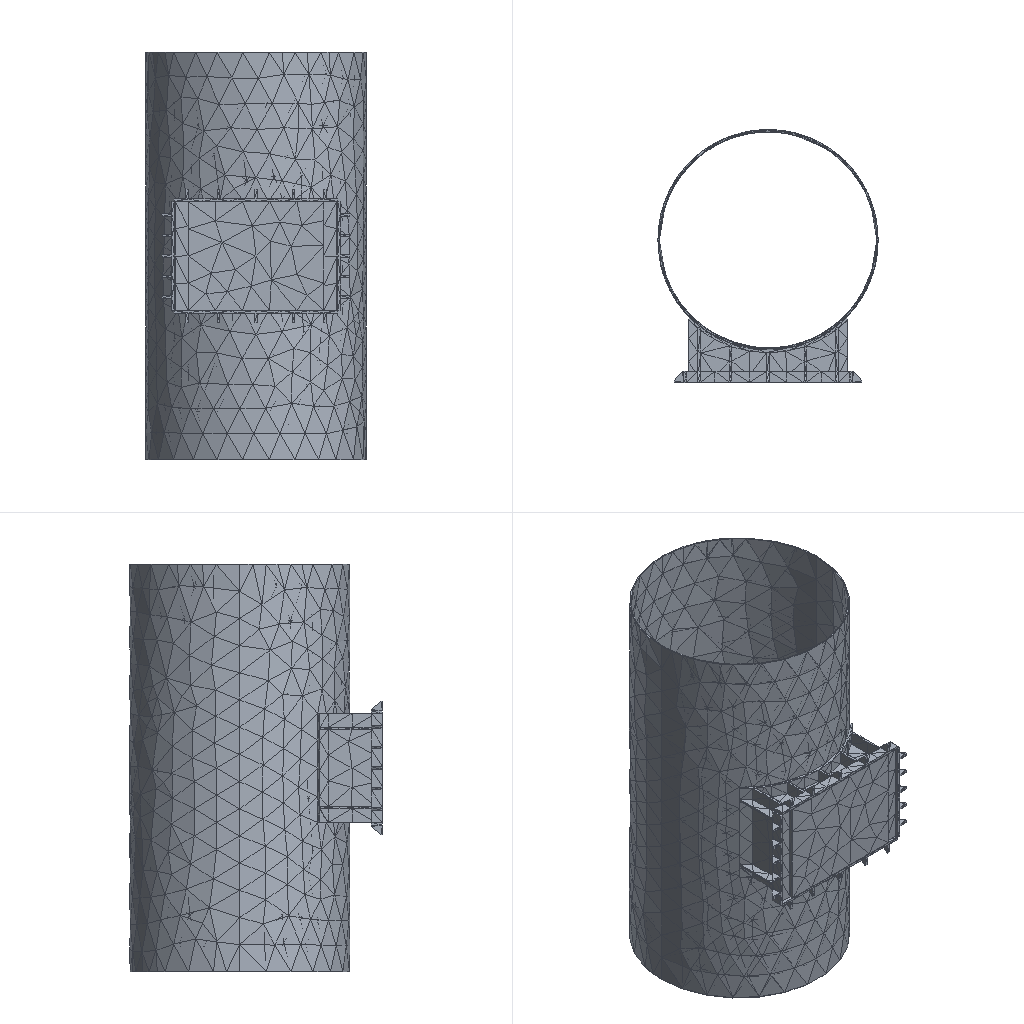Simulation study | ansys workbench
Set-up summary:
category,name,step,type,value,unit,region
solver,ansys_workbench
units,mm-N-s-tonne (MPa),,stated,"/units,MPA"
analysis,LS1,,static
load_step,LS1,LS1,static,nsubst=1; time=1
mesh,nodes,,,10077
mesh,elements,,,5774
element_type,SOLID187,,,4979
element_type,SURF154,,,571
element_type,TARGE170,,,112
element_type,CONTA174,,,112
material,q355,,E,200000,tonne s^-2 mm^-1
material,q355,,nu,0.3
material,q355,,density,7.85e-09,tonne mm^-3
material,q355,,conductivity,60.5,tonne mm s^-3 C^-1
material,q355,,specific_heat,4.34e+08,mm^2 s^-2 C^-1
material,q355,,cte,1.2e-05,C^-1
material,q355,,permeability,10000
material,q355,,resistivity,0.00017,ohm mm
load,Define Force Using Surface Effect Elements,LS1,surface-effect pres face 1,3.026,,SURF154 #8
load,Define Force Using Surface Effect Elements,LS1,surface-effect pres face 1,-3.026,,SURF154 #9
load,Define Force Using Surface Effect Elements,LS1,surface-effect pres face 2,-0.146,,SURF154 #10
load,Define Force Using Surface Effect Elements,LS1,surface-effect pres face 2,3.162,,SURF154 #11
load,Define Force Using Surface Effect Elements,LS1,surface-effect pres face 3,-1.925,,SURF154 #12
bc,Fixed Supports,model,fixed,[dofs=ALL],,_FIXEDSU
contact,Contact Region,,bonded (always),element=CONTA174
contact,Contact Region 2,,bonded (always),element=CONTA174
named_set,_FIXEDSU,,node,463
Ansys APDL input file, long lists of numbers shortened:
/batch
/config,noeldb,1     ! force off writing results to database
*get,_wallstrt,active,,time,wall
! ANSYS input file written by Workbench version 2022 R1
! File used for geometry attach:
/title,111--____ (B5)
! ****** Begin Custom Load Command Snippet ******
/COM, ACT Extensions:
/COM,     LSDYNA, 2021.1
/COM,
! ****** End   Custom Load Command Snippet ******
*DIM,_wb_ProjectScratch_dir,string,248
_wb_ProjectScratch_dir(1) = ''
*DIM,_wb_SolverFiles_dir,string,248
_wb_SolverFiles_dir(1) = ''
*DIM,_wb_userfiles_dir,string,248
_wb_userfiles_dir(1) = ''
/com,--- Data in consistent NMM units. See Solving Units in the help system for more information.
/units,MPA
/nopr
/wb,file,start              !  signify a WB generated input file
/prep7
! Turn off shape checking because checks already performed inside WB mesher.
! See help system for more information.
SHPP,OFF,,NOWARN
/nolist
etcon,set             ! allow ANSYS to choose best KEYOP's for 180x elements, resets any applicable keyopt to MAPDL defaults
/com,*********** Nodes for the whole assembly ***********
nblock,3,,11084
(1i9,3e20.9e3)
        1    -5.150000000E+02    -9.680000000E+02     4.200000000E+02
! (10076 more lines like these left out)
-1
/wb,elem,start            !  set before creation of elements
/com,*********** Elements for Body 1 "1-FreeParts|NONE" ***********
et,1,187
eblock,19,solid,,4736
(19i9)
        1        1        1        1        0        0        0        0       10        0      244     1292     2139     2144     1297     5916     9964     5917     5913
! (9471 more lines like these left out)
-1
/com,*********** Elements for Body 2 "1-FreeParts|__-__3" ***********
et,2,187
eblock,19,solid,,119
(19i9)
        2        2        2        2        0        0        0        0       10        0        1       12       14       65       16      149      170      154      150
! (237 more lines like these left out)
-1
/com,*********** Elements for Body 3 "1-FreeParts|__2" ***********
et,3,187
eblock,19,solid,,124
(19i9)
        3        3        3        3        0        0        0        0       10        0      120      363      411      410      419      523      687      522      524
! (247 more lines like these left out)
-1
/wb,elem,end               !  done creating elements
/com,*********** Send User Defined Coordinate System(s) ***********
csys,0
toffst,273.15,  ! Temperature offset from absolute zero
/com,*********** Set Reference Temperature ***********
tref,22.
/wb,mat,start              !  starting to send materials
/com,*********** Send Materials ***********
Temperature = 'TEMP' ! Temperature
MP,DENS,1,7.85e-09,	! tonne mm^-3
MP,ALPX,1,1.2e-05,	! C^-1
MP,C,1,434000000,	! mm^2 s^-2 C^-1
MP,KXX,1,60.5,	! tonne mm s^-3 C^-1
MP,RSVX,1,0.00017,	! ohm mm
MP,EX,1,200000,	! tonne s^-2 mm^-1
MP,NUXY,1,0.3,
MP,MURX,1,10000,
Temperature = 'TEMP' ! Temperature
MP,DENS,2,7.85e-09,	! tonne mm^-3
MP,ALPX,2,1.2e-05,	! C^-1
MP,C,2,434000000,	! mm^2 s^-2 C^-1
MP,KXX,2,60.5,	! tonne mm s^-3 C^-1
MP,RSVX,2,0.00017,	! ohm mm
MP,EX,2,200000,	! tonne s^-2 mm^-1
MP,NUXY,2,0.3,
MP,MURX,2,10000,
Temperature = 'TEMP' ! Temperature
MP,DENS,3,7.85e-09,	! tonne mm^-3
MP,ALPX,3,1.2e-05,	! C^-1
MP,C,3,434000000,	! mm^2 s^-2 C^-1
MP,KXX,3,60.5,	! tonne mm s^-3 C^-1
MP,RSVX,3,0.00017,	! ohm mm
MP,EX,3,200000,	! tonne s^-2 mm^-1
MP,NUXY,3,0.3,
MP,MURX,3,10000,
/wb,mat,end                !  done sending materials
!************************* Model Summary ********************
!1-FreeParts|NONE,	q355,	matid,	1
!1-FreeParts|__-__3,	q355,	matid,	2
!1-FreeParts|__2,	q355,	matid,	3
!************************* End Model Summary ********************
! get the diagonal of the bounding box. Needed later for other things
*get,_xmin,node,,mnloc,x
*get,_ymin,node,,mnloc,y
*get,_zmin,node,,mnloc,z
*get,_xmax,node,,mxloc,x
*get,_ymax,node,,mxloc,y
*get,_zmax,node,,mxloc,z
_ASMDIAG=(_xmax-_xmin)*(_xmax-_xmin)+(_ymax-_ymin)*(_ymax-_ymin)+(_zmax-_zmin)*(_zmax-_zmin)
_ASMDIAG=SQRT(_ASMDIAG)
/wb,contact,start          !  starting to send contact
/com,*********** Create Contact "接触区域" ***********
/com,            Real Constant Set For Above Contact Is 5 & 4
*set,tid,5
*set,cid,4
r,tid
r,cid
et,tid,170
et,cid,174
eblock,10,,,44
(15i9)
     8264        5        5        5        0      842     1090      874      874     3213     3332      874     3212
! (43 more lines like these left out)
-1
eblock,10,,,44
(15i9)
     8308        4        4        4        0      842     1090      874      874     3213     3332      874     3212
! (43 more lines like these left out)
-1
eblock,10,,,12
(15i9)
     8352        4        5        4        0       30       27       66       66      241      242       66      251
! (11 more lines like these left out)
-1
eblock,10,,,12
(15i9)
     8364        5        4        5        0       30       27       66       66      241      242       66      251
! (11 more lines like these left out)
-1
keyo,cid,8,2               ! auto create asymmetric contact (from Program Controlled setting)
keyo,cid,10,0              ! adjust contact stiffness each NR iteration (from Program Controlled setting)
keyo,cid,12,5              ! bonded always
keyo,cid,18,1              ! small sliding turned on by application
keyo,cid,2,0               ! augmented Lagrange (from Program Controlled setting)
keyo,cid,4,0               ! on Gauss point (from Program Controlled setting)
keyo,cid,9,1               ! ignore initial gaps/penetration
keyo,cid,7,0               ! No Prediction
rmod,tid,3,10.      ! FKN
rmod,tid,5,0.       ! ICONT
rmod,tid,6,0.       ! PINB
rmod,tid,10,0.      ! CNOF
rmod,tid,12,0.      ! FKT
rmod,tid,36,32      ! WB DSID
rmod,cid,3,10.      ! FKN
rmod,cid,5,0.       ! ICONT
rmod,cid,6,0.       ! PINB
rmod,cid,10,0.      ! CNOF
rmod,cid,12,0.      ! FKT
rmod,cid,36,32      ! WB DSID
/com,*********** Create Contact "接触区域 2" ***********
/com,            Real Constant Set For Above Contact Is 7 & 6
*set,tid,7
*set,cid,6
r,tid
r,cid
et,tid,170
et,cid,174
eblock,10,,,44
(15i9)
     8376        7        7        7        0      877     1199     1110     1110     3359     5061     1110     3358
! (43 more lines like these left out)
-1
eblock,10,,,44
(15i9)
     8420        6        6        6        0      877     1199     1110     1110     3359     5061     1110     3358
! (43 more lines like these left out)
-1
eblock,10,,,12
(15i9)
     8464        6        7        6        0      375      378      402      402      590      600      402      591
! (11 more lines like these left out)
-1
eblock,10,,,12
(15i9)
     8476        7        6        7        0      375      378      402      402      590      600      402      591
! (11 more lines like these left out)
-1
keyo,cid,8,2               ! auto create asymmetric contact (from Program Controlled setting)
keyo,cid,10,0              ! adjust contact stiffness each NR iteration (from Program Controlled setting)
keyo,cid,12,5              ! bonded always
keyo,cid,18,1              ! small sliding turned on by application
keyo,cid,2,0               ! augmented Lagrange (from Program Controlled setting)
keyo,cid,4,0               ! on Gauss point (from Program Controlled setting)
keyo,cid,9,1               ! ignore initial gaps/penetration
keyo,cid,7,0               ! No Prediction
rmod,tid,3,10.      ! FKN
rmod,tid,5,0.       ! ICONT
rmod,tid,6,0.       ! PINB
rmod,tid,10,0.      ! CNOF
rmod,tid,12,0.      ! FKT
rmod,tid,36,35      ! WB DSID
rmod,cid,3,10.      ! FKN
rmod,cid,5,0.       ! ICONT
rmod,cid,6,0.       ! PINB
rmod,cid,10,0.      ! CNOF
rmod,cid,12,0.      ! FKT
rmod,cid,36,35      ! WB DSID
nsel,all
esel,all
/wb,contact,end            !  done creating contacts
/golist
/wb,load,start             !  starting to send loads
/com,*********** Fixed Supports ***********
CMBLOCK,_FIXEDSU,NODE,      463
(8i10)
         2         4         5         7         8        11        13        14
! (57 more lines like these left out)
cmsel,s,_FIXEDSU
d,all,all
nsel,all
/com,*********** Define Force Using Surface Effect Elements ***********
local,12,0,0.,0.,0.,0.,0.,0.
csys,0
et,8,154
eblock,10,,,14
(15i9)
     8488        8        8        8       12     1100     2154     2153     2153     5015     9987     2153     5014
! (13 more lines like these left out)
-1
esel,s,type,,8
keyop,8,2,1                ! Apply load in local coordinate system
keyop,8,7,1                ! Use original area so load is constant in large deformation
esel,all
/com,*********** Define Force Using Surface Effect Elements ***********
local,13,0,0.,0.,0.,0.,0.,0.
csys,0
et,9,154
eblock,10,,,14
(15i9)
     8502        9        9        9       13     1079     1080     2151     2151     4860     4877     2151     4866
! (13 more lines like these left out)
-1
esel,s,type,,9
keyop,9,2,1                ! Apply load in local coordinate system
keyop,9,7,1                ! Use original area so load is constant in large deformation
esel,all
/com,*********** Define Force Using Surface Effect Elements ***********
local,14,0,0.,0.,0.,0.,0.,0.
csys,0
et,10,154
eblock,10,,,437
(15i9)
     8516       10       10       10       14      718     2089      732      732     2364     2500      732     2361
! (436 more lines like these left out)
-1
esel,s,type,,10
keyop,10,2,1                ! Apply load in local coordinate system
keyop,10,7,1                ! Use original area so load is constant in large deformation
esel,all
/com,*********** Define Force Using Surface Effect Elements ***********
local,15,0,0.,0.,0.,0.,0.,0.
csys,0
et,11,154
eblock,10,,,74
(15i9)
     8953       11       11       11       15     1372     1105     1101     1101     5040     5017     1101     5020
! (73 more lines like these left out)
-1
esel,s,type,,11
keyop,11,2,1                ! Apply load in local coordinate system
keyop,11,7,1                ! Use original area so load is constant in large deformation
esel,all
/com,*********** Define Force Using Surface Effect Elements ***********
local,16,0,0.,0.,0.,0.,0.,0.
csys,0
et,12,154
eblock,10,,,32
(15i9)
     9027       12       12       12       16      994     1023     1043     1043     4343     4541     1043     4344
! (31 more lines like these left out)
-1
esel,s,type,,12
keyop,12,2,1                ! Apply load in local coordinate system
keyop,12,7,1                ! Use original area so load is constant in large deformation
esel,all
/gst,on,on
fini
*get,_numnode,node,0,count
*get,_numelem,elem,0,count
*get, _MAXELEMNUM, elem, 0, NUM, MAX
*get, _MAXNODENUM, node, 0, NUM, MAX
*get, _MAXELEMTYPE, etyp, 0, NUM, MAX
*get, _MAXREALCONST, real, 0, NUM, MAX
/go
/wb,load,end               !  done creating loads
/com,--- Number of total nodes = %_numnode%
/com,--- Number of contact elements = 795
/com,--- Number of spring elements = 0
/com,--- Number of bearing elements = 0
/com,--- Number of solid elements = 4979
/com,--- Number of condensed parts = 0
/com,--- Number of total elements = %_numelem%
*get,_wallbsol,active,,time,wall
/com,****************************************************************************
/com,*************************    SOLUTION       ********************************
/com,****************************************************************************
/solu
antype,0                   ! static analysis
_thickRatio=  0     ! Ratio of thick parts in the model
eqsl,sparse,,,,,1
cntr,print,1               ! print out contact info and also make no initial contact an error
dmpoption,emat,no             ! Don't combine emat file for DANSYS
dmpoption,esav,no             ! Don't combine esav file for DANSYS
nldiag,cont,iter           ! print out contact info each equilibrium iteration
rescontrol,,none                 ! Do not keep any restart files
/com,****************************************************
/com,******************* SOLVE FOR LS 1 OF 1 ****************
esel,s,type,,8
nsle
sfe,all,1,pres,1,3.026
sfe,all,2,pres,1,0.
sfe,all,3,pres,1,0.
esel,s,type,,9
nsle
sfe,all,1,pres,1,-3.026
sfe,all,2,pres,1,0.
sfe,all,3,pres,1,0.
esel,s,type,,10
nsle
sfe,all,1,pres,1,0.
sfe,all,2,pres,1,-0.146
sfe,all,3,pres,1,0.
esel,s,type,,11
nsle
sfe,all,1,pres,1,0.
sfe,all,2,pres,1,3.162
sfe,all,3,pres,1,0.
esel,s,type,,12
nsle
sfe,all,1,pres,1,0.
sfe,all,2,pres,1,0.
sfe,all,3,pres,1,-1.925
nsel,all
esel,all
/nopr
/gopr
nsub,1,1,1
time,1.
outres,erase
outres,all,none
outres,nsol,all,
outres,rsol,all
outres,eangl,all
outres,etmp,all
outres,veng,all
outres,strs,all,
outres,epel,all,
outres,eppl,all,
outres,cont,all,
! *********** WB SOLVE COMMAND ***********
! check interactive state
*get,ANSINTER_,active,,int
*if,ANSINTER_,ne,0,then
/eof
*endif
solve
/com *************** Write FE CONNECTORS *********
CEWRITE,file,ce,,INTE
/com,****************************************************
/com,*************** FINISHED SOLVE FOR LS 1 *************
*get,_wallasol,active,,time,wall
/nopr
*get,_numnode,node,0,count
*get,_numelem,elem,0,count
*get, _MAXELEMNUM, elem, 0, NUM, MAX
*get, _MAXNODENUM, node, 0, NUM, MAX,,,INTERNAL
*get, _MAXELEMTYPE, etyp, 0, NUM, MAX
*get, _MAXREALCONST, real, 0, NUM, MAX
/gopr
/post1
xmlo,ENCODING,ISO-8859-1
xmlo,parm
/xml,parm,xml
fini
/gopr
*get,_walldone,active,,time,wall
_preptime=(_wallbsol-_wallstrt)*3600
_solvtime=(_wallasol-_wallbsol)*3600
_posttime=(_walldone-_wallasol)*3600
_totaltim=(_walldone-_wallstrt)*3600
*get,_dlbratio,active,0,solu,dlbr
*get,_combtime,active,0,solu,comb
*get,_ssmode,active,0,solu,ssmm
*get,_ndofs,active,0,solu,ndof
*get,_sol_end_time,active,0,set,time
*if,_sol_end_time,eq,1.,then
/fclean				!clean distributed files
*endif
/com,--- Total number of nodes = %_numnode%
/com,--- Total number of elements = %_numelem%
/com,--- Element load balance ratio = %_dlbratio%
/com,--- Time to combine distributed files = %_combtime%
/com,--- Sparse memory mode = %_ssmode%
/com,--- Number of DOF = %_ndofs%
/wb,file,end               ! done with WB generated input
Results summary:
result,analyses[0].index,,,1
result,analyses[0].system,,,SYS
result,analyses[0].deck,,,deck.dat
result,analyses[0].solve_status,,,completed
result,analyses[0].analysis_type,,,static
result,analyses[0].physics,,,mechanical
result,analyses[0].unit_system,,,"NMM: mm, ton, N, s, mV, mA, degC"
result,analyses[0].n_sets,,,1
result,analyses[0].load_steps[0].set,set=1,,1
result,analyses[0].load_steps[0].time_or_freq,set=1,,1
result,analyses[0].load_steps[0].max_displacement_magnitude,set=1,,3.656
result,analyses[0].load_steps[0].max_von_mises_nodal,set=1,,118.911
result,analyses[0].load_steps[0].reaction_force_sum_xyz[1],set=1,,-3.98429e-06
result,analyses[0].load_steps[0].reaction_force_sum_xyz[2],set=1,,-0.2158
result,analyses[0].load_steps[0].reaction_force_sum_xyz[3],set=1,,500000